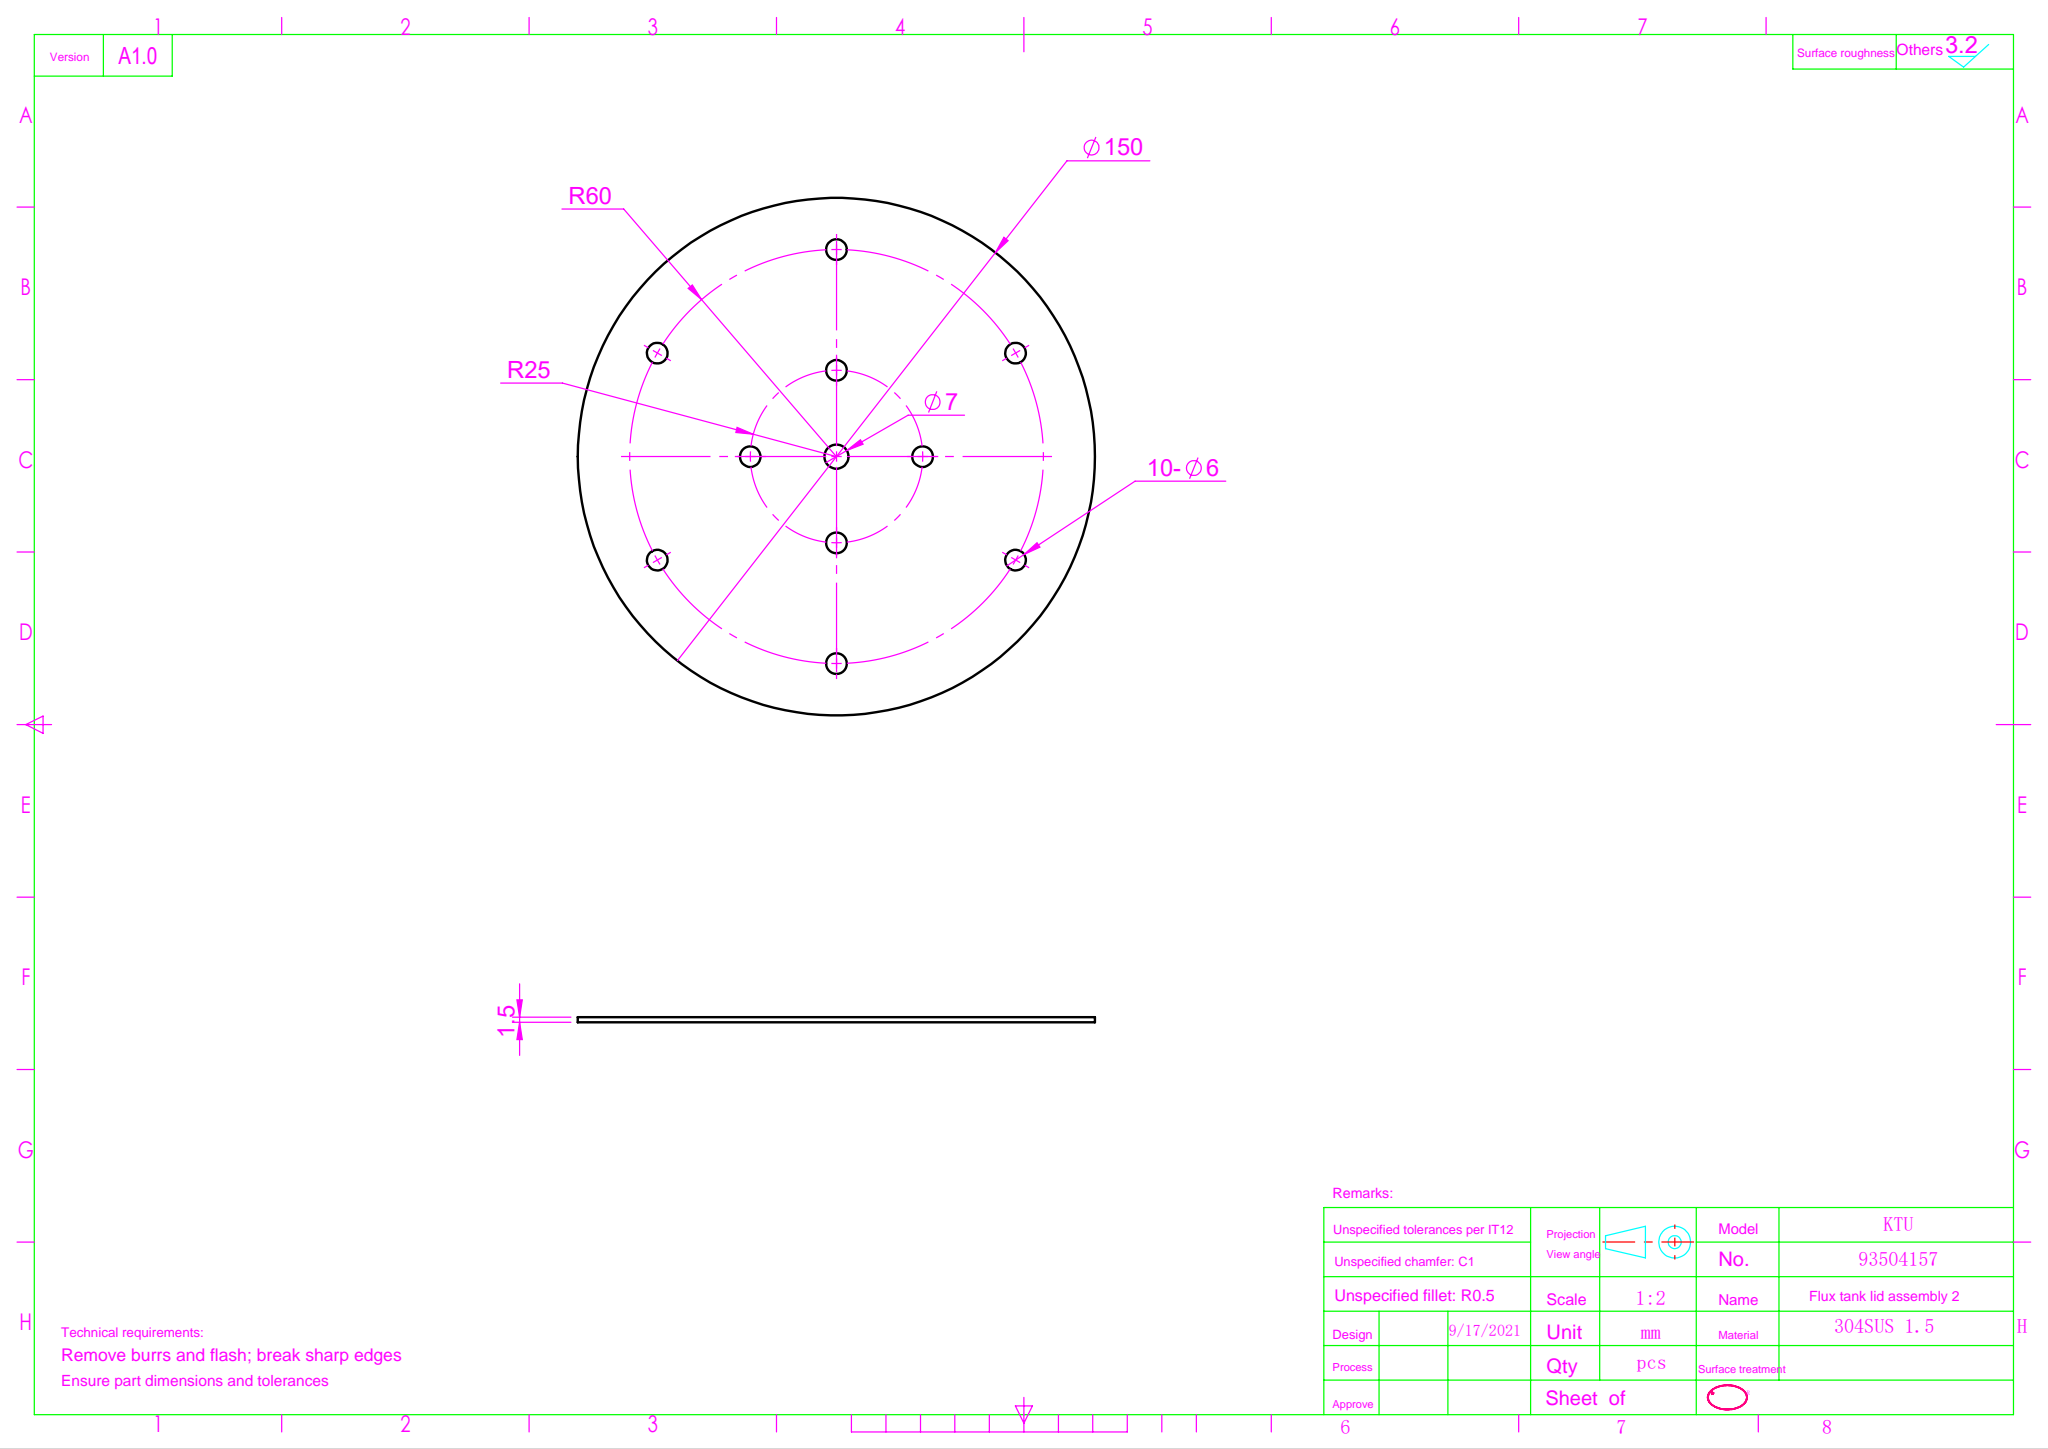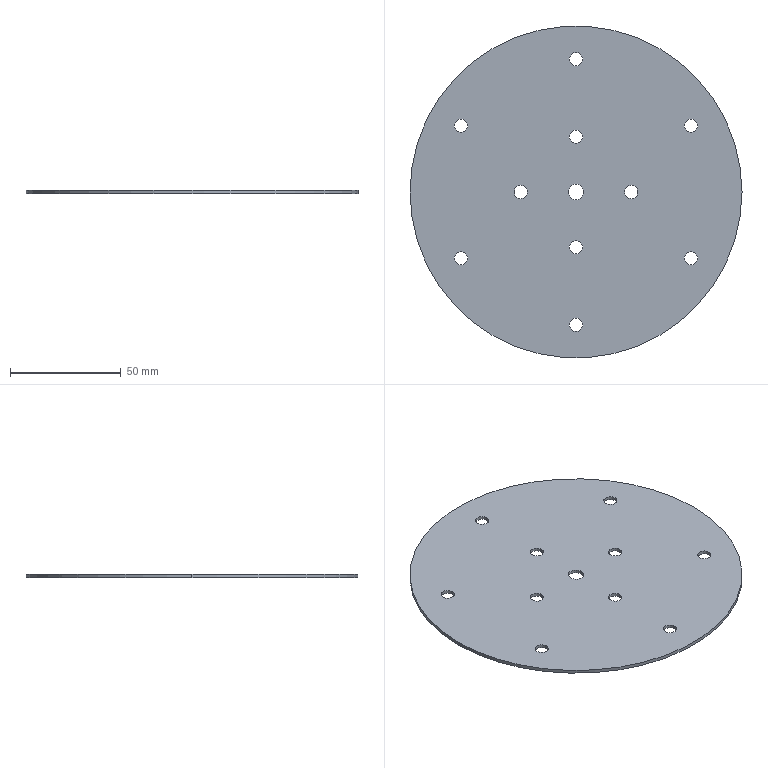Part | SolidWorks | features CirPattern 2, ICE 2, FlatPattern 1, HoleWzd 1, SMBaseFlange 1, SheetMetal 1 | 1 solid | 26 faces | box 150 x 150 x 1.5 mm | volume 26025 mm3 | cylinder 24 | plane 2 | commonest cylinder face diameters 6 x20 7 x2 150 x2
STEP:
#1=CARTESIAN_POINT('',(28.,0.,0.));
#2=VERTEX_POINT('',#1);
#3=CARTESIAN_POINT('',(22.,0.,0.));
#4=VERTEX_POINT('',#3);
#5=CARTESIAN_POINT('',(25.,0.,0.));
#6=DIRECTION('',(0.,0.,-1.));
#7=DIRECTION('',(1.,0.,0.));
#8=AXIS2_PLACEMENT_3D('',#5,#6,#7);
#9=CIRCLE('',#8,3.);
#10=EDGE_CURVE('',#2,#4,#9,.T.);
#11=ORIENTED_EDGE('',*,*,#10,.F.);
#12=CARTESIAN_POINT('',(28.,0.,-1.5));
#13=VERTEX_POINT('',#12);
#14=CARTESIAN_POINT('',(28.,0.,0.));
#15=DIRECTION('',(0.,0.,-1.));
#16=VECTOR('',#15,1000.);
#17=LINE('',#14,#16);
#18=EDGE_CURVE('',#2,#13,#17,.T.);
#19=ORIENTED_EDGE('',*,*,#18,.T.);
#20=CARTESIAN_POINT('',(22.,0.,-1.5));
#21=VERTEX_POINT('',#20);
#22=CARTESIAN_POINT('',(25.,0.,-1.5));
#23=DIRECTION('',(0.,0.,-1.));
#24=DIRECTION('',(1.,0.,0.));
#25=AXIS2_PLACEMENT_3D('',#22,#23,#24);
#26=CIRCLE('',#25,3.);
#27=EDGE_CURVE('',#13,#21,#26,.T.);
#28=ORIENTED_EDGE('',*,*,#27,.T.);
#29=CARTESIAN_POINT('',(22.,0.,0.));
#30=DIRECTION('',(0.,0.,-1.));
#31=VECTOR('',#30,1000.);
#32=LINE('',#29,#31);
#33=EDGE_CURVE('',#4,#21,#32,.T.);
#34=ORIENTED_EDGE('',*,*,#33,.F.);
#35=EDGE_LOOP('',(#11,#19,#28,#34));
#36=FACE_OUTER_BOUND('',#35,.T.);
#37=CARTESIAN_POINT('',(25.,0.,0.));
#38=DIRECTION('',(0.,0.,-1.));
#39=DIRECTION('',(-1.,0.,0.));
#40=AXIS2_PLACEMENT_3D('',#37,#38,#39);
#41=CYLINDRICAL_SURFACE('',#40,3.);
#42=ADVANCED_FACE('',(#36),#41,.F.);
#43=CARTESIAN_POINT('',(3.,25.,0.));
#44=VERTEX_POINT('',#43);
#45=CARTESIAN_POINT('',(-3.,25.,0.));
#46=VERTEX_POINT('',#45);
#47=CARTESIAN_POINT('',(0.,25.,0.));
#48=DIRECTION('',(0.,0.,-1.));
#49=DIRECTION('',(0.,1.,0.));
#50=AXIS2_PLACEMENT_3D('',#47,#48,#49);
#51=CIRCLE('',#50,3.);
#52=EDGE_CURVE('',#44,#46,#51,.T.);
#53=ORIENTED_EDGE('',*,*,#52,.F.);
#54=CARTESIAN_POINT('',(3.,25.,-1.5));
#55=VERTEX_POINT('',#54);
#56=CARTESIAN_POINT('',(3.,25.,0.));
#57=DIRECTION('',(0.,0.,-1.));
#58=VECTOR('',#57,1000.);
#59=LINE('',#56,#58);
#60=EDGE_CURVE('',#44,#55,#59,.T.);
#61=ORIENTED_EDGE('',*,*,#60,.T.);
#62=CARTESIAN_POINT('',(-3.,25.,-1.5));
#63=VERTEX_POINT('',#62);
#64=CARTESIAN_POINT('',(0.,25.,-1.5));
#65=DIRECTION('',(0.,0.,-1.));
#66=DIRECTION('',(0.,1.,0.));
#67=AXIS2_PLACEMENT_3D('',#64,#65,#66);
#68=CIRCLE('',#67,3.);
#69=EDGE_CURVE('',#55,#63,#68,.T.);
#70=ORIENTED_EDGE('',*,*,#69,.T.);
#71=CARTESIAN_POINT('',(-3.,25.,0.));
#72=DIRECTION('',(0.,0.,-1.));
#73=VECTOR('',#72,1000.);
#74=LINE('',#71,#73);
#75=EDGE_CURVE('',#46,#63,#74,.T.);
#76=ORIENTED_EDGE('',*,*,#75,.F.);
#77=EDGE_LOOP('',(#53,#61,#70,#76));
#78=FACE_OUTER_BOUND('',#77,.T.);
#79=CARTESIAN_POINT('',(0.,25.,0.));
#80=DIRECTION('',(0.,0.,-1.));
#81=DIRECTION('',(-1.,0.,0.));
#82=AXIS2_PLACEMENT_3D('',#79,#80,#81);
#83=CYLINDRICAL_SURFACE('',#82,3.);
#84=ADVANCED_FACE('',(#78),#83,.F.);
#85=CARTESIAN_POINT('',(3.,-25.,0.));
#86=VERTEX_POINT('',#85);
#87=CARTESIAN_POINT('',(-3.,-25.,0.));
#88=VERTEX_POINT('',#87);
#89=CARTESIAN_POINT('',(0.,-25.,0.));
#90=DIRECTION('',(0.,0.,-1.));
#91=DIRECTION('',(0.,-1.,0.));
#92=AXIS2_PLACEMENT_3D('',#89,#90,#91);
#93=CIRCLE('',#92,3.);
#94=EDGE_CURVE('',#86,#88,#93,.T.);
#95=ORIENTED_EDGE('',*,*,#94,.F.);
#96=CARTESIAN_POINT('',(3.,-25.,-1.5));
#97=VERTEX_POINT('',#96);
#98=CARTESIAN_POINT('',(3.,-25.,0.));
#99=DIRECTION('',(0.,0.,-1.));
#100=VECTOR('',#99,1000.);
#101=LINE('',#98,#100);
#102=EDGE_CURVE('',#86,#97,#101,.T.);
#103=ORIENTED_EDGE('',*,*,#102,.T.);
#104=CARTESIAN_POINT('',(-3.,-25.,-1.5));
#105=VERTEX_POINT('',#104);
#106=CARTESIAN_POINT('',(0.,-25.,-1.5));
#107=DIRECTION('',(0.,0.,-1.));
#108=DIRECTION('',(0.,-1.,0.));
#109=AXIS2_PLACEMENT_3D('',#106,#107,#108);
#110=CIRCLE('',#109,3.);
#111=EDGE_CURVE('',#97,#105,#110,.T.);
#112=ORIENTED_EDGE('',*,*,#111,.T.);
#113=CARTESIAN_POINT('',(-3.,-25.,0.));
#114=DIRECTION('',(0.,0.,-1.));
#115=VECTOR('',#114,1000.);
#116=LINE('',#113,#115);
#117=EDGE_CURVE('',#88,#105,#116,.T.);
#118=ORIENTED_EDGE('',*,*,#117,.F.);
#119=EDGE_LOOP('',(#95,#103,#112,#118));
#120=FACE_OUTER_BOUND('',#119,.T.);
#121=CARTESIAN_POINT('',(0.,-25.,0.));
#122=DIRECTION('',(0.,0.,-1.));
#123=DIRECTION('',(-1.,0.,0.));
#124=AXIS2_PLACEMENT_3D('',#121,#122,#123);
#125=CYLINDRICAL_SURFACE('',#124,3.);
#126=ADVANCED_FACE('',(#120),#125,.F.);
#127=CARTESIAN_POINT('',(-22.,0.,0.));
#128=VERTEX_POINT('',#127);
#129=CARTESIAN_POINT('',(-28.,0.,0.));
#130=VERTEX_POINT('',#129);
#131=CARTESIAN_POINT('',(-25.,0.,0.));
#132=DIRECTION('',(0.,0.,-1.));
#133=DIRECTION('',(-1.,0.,0.));
#134=AXIS2_PLACEMENT_3D('',#131,#132,#133);
#135=CIRCLE('',#134,3.);
#136=EDGE_CURVE('',#128,#130,#135,.T.);
#137=ORIENTED_EDGE('',*,*,#136,.F.);
#138=CARTESIAN_POINT('',(-22.,0.,-1.5));
#139=VERTEX_POINT('',#138);
#140=CARTESIAN_POINT('',(-22.,0.,0.));
#141=DIRECTION('',(0.,0.,-1.));
#142=VECTOR('',#141,1000.);
#143=LINE('',#140,#142);
#144=EDGE_CURVE('',#128,#139,#143,.T.);
#145=ORIENTED_EDGE('',*,*,#144,.T.);
#146=CARTESIAN_POINT('',(-28.,0.,-1.5));
#147=VERTEX_POINT('',#146);
#148=CARTESIAN_POINT('',(-25.,0.,-1.5));
#149=DIRECTION('',(0.,0.,-1.));
#150=DIRECTION('',(-1.,0.,0.));
#151=AXIS2_PLACEMENT_3D('',#148,#149,#150);
#152=CIRCLE('',#151,3.);
#153=EDGE_CURVE('',#139,#147,#152,.T.);
#154=ORIENTED_EDGE('',*,*,#153,.T.);
#155=CARTESIAN_POINT('',(-28.,0.,0.));
#156=DIRECTION('',(0.,0.,-1.));
#157=VECTOR('',#156,1000.);
#158=LINE('',#155,#157);
#159=EDGE_CURVE('',#130,#147,#158,.T.);
#160=ORIENTED_EDGE('',*,*,#159,.F.);
#161=EDGE_LOOP('',(#137,#145,#154,#160));
#162=FACE_OUTER_BOUND('',#161,.T.);
#163=CARTESIAN_POINT('',(-25.,0.,0.));
#164=DIRECTION('',(0.,0.,-1.));
#165=DIRECTION('',(-1.,0.,0.));
#166=AXIS2_PLACEMENT_3D('',#163,#164,#165);
#167=CYLINDRICAL_SURFACE('',#166,3.);
#168=ADVANCED_FACE('',(#162),#167,.F.);
#169=CARTESIAN_POINT('',(-48.962,-30.,0.));
#170=VERTEX_POINT('',#169);
#171=CARTESIAN_POINT('',(-54.962,-30.,0.));
#172=VERTEX_POINT('',#171);
#173=CARTESIAN_POINT('',(-51.962,-30.,0.));
#174=DIRECTION('',(0.,0.,-1.));
#175=DIRECTION('',(1.,0.,0.));
#176=AXIS2_PLACEMENT_3D('',#173,#174,#175);
#177=CIRCLE('',#176,3.);
#178=EDGE_CURVE('',#170,#172,#177,.T.);
#179=ORIENTED_EDGE('',*,*,#178,.F.);
#180=CARTESIAN_POINT('',(-48.962,-30.,-1.5));
#181=VERTEX_POINT('',#180);
#182=CARTESIAN_POINT('',(-48.962,-30.,0.001));
#183=DIRECTION('',(0.,0.,-1.));
#184=VECTOR('',#183,1000.);
#185=LINE('',#182,#184);
#186=EDGE_CURVE('',#170,#181,#185,.T.);
#187=ORIENTED_EDGE('',*,*,#186,.T.);
#188=CARTESIAN_POINT('',(-54.962,-30.,-1.5));
#189=VERTEX_POINT('',#188);
#190=CARTESIAN_POINT('',(-51.962,-30.,-1.5));
#191=DIRECTION('',(0.,0.,-1.));
#192=DIRECTION('',(0.5,-0.866,0.));
#193=AXIS2_PLACEMENT_3D('',#190,#191,#192);
#194=CIRCLE('',#193,3.);
#195=EDGE_CURVE('',#181,#189,#194,.T.);
#196=ORIENTED_EDGE('',*,*,#195,.T.);
#197=CARTESIAN_POINT('',(-54.962,-30.,0.001));
#198=DIRECTION('',(0.,0.,-1.));
#199=VECTOR('',#198,1000.);
#200=LINE('',#197,#199);
#201=EDGE_CURVE('',#172,#189,#200,.T.);
#202=ORIENTED_EDGE('',*,*,#201,.F.);
#203=EDGE_LOOP('',(#179,#187,#196,#202));
#204=FACE_OUTER_BOUND('',#203,.T.);
#205=CARTESIAN_POINT('',(-51.962,-30.,0.001));
#206=DIRECTION('',(0.,0.,-1.));
#207=DIRECTION('',(-1.,0.,0.));
#208=AXIS2_PLACEMENT_3D('',#205,#206,#207);
#209=CYLINDRICAL_SURFACE('',#208,3.);
#210=ADVANCED_FACE('',(#204),#209,.F.);
#211=CARTESIAN_POINT('',(3.,-60.,0.));
#212=VERTEX_POINT('',#211);
#213=CARTESIAN_POINT('',(-3.,-60.,0.));
#214=VERTEX_POINT('',#213);
#215=CARTESIAN_POINT('',(0.,-60.,0.));
#216=DIRECTION('',(0.,0.,-1.));
#217=DIRECTION('',(1.,0.,0.));
#218=AXIS2_PLACEMENT_3D('',#215,#216,#217);
#219=CIRCLE('',#218,3.);
#220=EDGE_CURVE('',#212,#214,#219,.T.);
#221=ORIENTED_EDGE('',*,*,#220,.F.);
#222=CARTESIAN_POINT('',(3.,-60.,-1.5));
#223=VERTEX_POINT('',#222);
#224=CARTESIAN_POINT('',(3.,-60.,0.001));
#225=DIRECTION('',(0.,0.,-1.));
#226=VECTOR('',#225,1000.);
#227=LINE('',#224,#226);
#228=EDGE_CURVE('',#212,#223,#227,.T.);
#229=ORIENTED_EDGE('',*,*,#228,.T.);
#230=CARTESIAN_POINT('',(-3.,-60.,-1.5));
#231=VERTEX_POINT('',#230);
#232=CARTESIAN_POINT('',(0.,-60.,-1.5));
#233=DIRECTION('',(0.,0.,-1.));
#234=DIRECTION('',(1.,0.,0.));
#235=AXIS2_PLACEMENT_3D('',#232,#233,#234);
#236=CIRCLE('',#235,3.);
#237=EDGE_CURVE('',#223,#231,#236,.T.);
#238=ORIENTED_EDGE('',*,*,#237,.T.);
#239=CARTESIAN_POINT('',(-3.,-60.,0.001));
#240=DIRECTION('',(0.,0.,-1.));
#241=VECTOR('',#240,1000.);
#242=LINE('',#239,#241);
#243=EDGE_CURVE('',#214,#231,#242,.T.);
#244=ORIENTED_EDGE('',*,*,#243,.F.);
#245=EDGE_LOOP('',(#221,#229,#238,#244));
#246=FACE_OUTER_BOUND('',#245,.T.);
#247=CARTESIAN_POINT('',(0.,-60.,0.001));
#248=DIRECTION('',(0.,0.,-1.));
#249=DIRECTION('',(-1.,0.,0.));
#250=AXIS2_PLACEMENT_3D('',#247,#248,#249);
#251=CYLINDRICAL_SURFACE('',#250,3.);
#252=ADVANCED_FACE('',(#246),#251,.F.);
#253=CARTESIAN_POINT('',(54.962,-30.,0.));
#254=VERTEX_POINT('',#253);
#255=CARTESIAN_POINT('',(48.962,-30.,0.));
#256=VERTEX_POINT('',#255);
#257=CARTESIAN_POINT('',(51.962,-30.,0.));
#258=DIRECTION('',(0.,0.,-1.));
#259=DIRECTION('',(1.,0.,0.));
#260=AXIS2_PLACEMENT_3D('',#257,#258,#259);
#261=CIRCLE('',#260,3.);
#262=EDGE_CURVE('',#254,#256,#261,.T.);
#263=ORIENTED_EDGE('',*,*,#262,.F.);
#264=CARTESIAN_POINT('',(54.962,-30.,-1.5));
#265=VERTEX_POINT('',#264);
#266=CARTESIAN_POINT('',(54.962,-30.,0.001));
#267=DIRECTION('',(0.,0.,-1.));
#268=VECTOR('',#267,1000.);
#269=LINE('',#266,#268);
#270=EDGE_CURVE('',#254,#265,#269,.T.);
#271=ORIENTED_EDGE('',*,*,#270,.T.);
#272=CARTESIAN_POINT('',(48.962,-30.,-1.5));
#273=VERTEX_POINT('',#272);
#274=CARTESIAN_POINT('',(51.962,-30.,-1.5));
#275=DIRECTION('',(0.,0.,-1.));
#276=DIRECTION('',(0.5,0.866,0.));
#277=AXIS2_PLACEMENT_3D('',#274,#275,#276);
#278=CIRCLE('',#277,3.);
#279=EDGE_CURVE('',#265,#273,#278,.T.);
#280=ORIENTED_EDGE('',*,*,#279,.T.);
#281=CARTESIAN_POINT('',(48.962,-30.,0.001));
#282=DIRECTION('',(0.,0.,-1.));
#283=VECTOR('',#282,1000.);
#284=LINE('',#281,#283);
#285=EDGE_CURVE('',#256,#273,#284,.T.);
#286=ORIENTED_EDGE('',*,*,#285,.F.);
#287=EDGE_LOOP('',(#263,#271,#280,#286));
#288=FACE_OUTER_BOUND('',#287,.T.);
#289=CARTESIAN_POINT('',(51.962,-30.,0.001));
#290=DIRECTION('',(0.,0.,-1.));
#291=DIRECTION('',(-1.,0.,0.));
#292=AXIS2_PLACEMENT_3D('',#289,#290,#291);
#293=CYLINDRICAL_SURFACE('',#292,3.);
#294=ADVANCED_FACE('',(#288),#293,.F.);
#295=CARTESIAN_POINT('',(54.962,30.,0.));
#296=VERTEX_POINT('',#295);
#297=CARTESIAN_POINT('',(48.962,30.,0.));
#298=VERTEX_POINT('',#297);
#299=CARTESIAN_POINT('',(51.962,30.,0.));
#300=DIRECTION('',(0.,0.,-1.));
#301=DIRECTION('',(1.,0.,0.));
#302=AXIS2_PLACEMENT_3D('',#299,#300,#301);
#303=CIRCLE('',#302,3.);
#304=EDGE_CURVE('',#296,#298,#303,.T.);
#305=ORIENTED_EDGE('',*,*,#304,.F.);
#306=CARTESIAN_POINT('',(54.962,30.,-1.5));
#307=VERTEX_POINT('',#306);
#308=CARTESIAN_POINT('',(54.962,30.,0.001));
#309=DIRECTION('',(0.,0.,-1.));
#310=VECTOR('',#309,1000.);
#311=LINE('',#308,#310);
#312=EDGE_CURVE('',#296,#307,#311,.T.);
#313=ORIENTED_EDGE('',*,*,#312,.T.);
#314=CARTESIAN_POINT('',(48.962,30.,-1.5));
#315=VERTEX_POINT('',#314);
#316=CARTESIAN_POINT('',(51.962,30.,-1.5));
#317=DIRECTION('',(0.,0.,-1.));
#318=DIRECTION('',(-0.5,0.866,0.));
#319=AXIS2_PLACEMENT_3D('',#316,#317,#318);
#320=CIRCLE('',#319,3.);
#321=EDGE_CURVE('',#307,#315,#320,.T.);
#322=ORIENTED_EDGE('',*,*,#321,.T.);
#323=CARTESIAN_POINT('',(48.962,30.,0.001));
#324=DIRECTION('',(0.,0.,-1.));
#325=VECTOR('',#324,1000.);
#326=LINE('',#323,#325);
#327=EDGE_CURVE('',#298,#315,#326,.T.);
#328=ORIENTED_EDGE('',*,*,#327,.F.);
#329=EDGE_LOOP('',(#305,#313,#322,#328));
#330=FACE_OUTER_BOUND('',#329,.T.);
#331=CARTESIAN_POINT('',(51.962,30.,0.001));
#332=DIRECTION('',(0.,0.,-1.));
#333=DIRECTION('',(-1.,0.,0.));
#334=AXIS2_PLACEMENT_3D('',#331,#332,#333);
#335=CYLINDRICAL_SURFACE('',#334,3.);
#336=ADVANCED_FACE('',(#330),#335,.F.);
#337=CARTESIAN_POINT('',(-48.962,30.,0.));
#338=VERTEX_POINT('',#337);
#339=CARTESIAN_POINT('',(-54.962,30.,0.));
#340=VERTEX_POINT('',#339);
#341=CARTESIAN_POINT('',(-51.962,30.,0.));
#342=DIRECTION('',(0.,0.,-1.));
#343=DIRECTION('',(1.,0.,0.));
#344=AXIS2_PLACEMENT_3D('',#341,#342,#343);
#345=CIRCLE('',#344,3.);
#346=EDGE_CURVE('',#338,#340,#345,.T.);
#347=ORIENTED_EDGE('',*,*,#346,.F.);
#348=CARTESIAN_POINT('',(-48.962,30.,-1.5));
#349=VERTEX_POINT('',#348);
#350=CARTESIAN_POINT('',(-48.962,30.,0.001));
#351=DIRECTION('',(0.,0.,-1.));
#352=VECTOR('',#351,1000.);
#353=LINE('',#350,#352);
#354=EDGE_CURVE('',#338,#349,#353,.T.);
#355=ORIENTED_EDGE('',*,*,#354,.T.);
#356=CARTESIAN_POINT('',(-54.962,30.,-1.5));
#357=VERTEX_POINT('',#356);
#358=CARTESIAN_POINT('',(-51.962,30.,-1.5));
#359=DIRECTION('',(0.,0.,-1.));
#360=DIRECTION('',(-0.5,-0.866,0.));
#361=AXIS2_PLACEMENT_3D('',#358,#359,#360);
#362=CIRCLE('',#361,3.);
#363=EDGE_CURVE('',#349,#357,#362,.T.);
#364=ORIENTED_EDGE('',*,*,#363,.T.);
#365=CARTESIAN_POINT('',(-54.962,30.,0.001));
#366=DIRECTION('',(0.,0.,-1.));
#367=VECTOR('',#366,1000.);
#368=LINE('',#365,#367);
#369=EDGE_CURVE('',#340,#357,#368,.T.);
#370=ORIENTED_EDGE('',*,*,#369,.F.);
#371=EDGE_LOOP('',(#347,#355,#364,#370));
#372=FACE_OUTER_BOUND('',#371,.T.);
#373=CARTESIAN_POINT('',(-51.962,30.,0.001));
#374=DIRECTION('',(0.,0.,-1.));
#375=DIRECTION('',(-1.,0.,0.));
#376=AXIS2_PLACEMENT_3D('',#373,#374,#375);
#377=CYLINDRICAL_SURFACE('',#376,3.);
#378=ADVANCED_FACE('',(#372),#377,.F.);
#379=CARTESIAN_POINT('',(3.,60.,0.));
#380=VERTEX_POINT('',#379);
#381=CARTESIAN_POINT('',(-3.,60.,0.));
#382=VERTEX_POINT('',#381);
#383=CARTESIAN_POINT('',(0.,60.,0.));
#384=DIRECTION('',(0.,0.,-1.));
#385=DIRECTION('',(1.,0.,0.));
#386=AXIS2_PLACEMENT_3D('',#383,#384,#385);
#387=CIRCLE('',#386,3.);
#388=EDGE_CURVE('',#380,#382,#387,.T.);
#389=ORIENTED_EDGE('',*,*,#388,.F.);
#390=CARTESIAN_POINT('',(3.,60.,-1.5));
#391=VERTEX_POINT('',#390);
#392=CARTESIAN_POINT('',(3.,60.,0.001));
#393=DIRECTION('',(0.,0.,-1.));
#394=VECTOR('',#393,1000.);
#395=LINE('',#392,#394);
#396=EDGE_CURVE('',#380,#391,#395,.T.);
#397=ORIENTED_EDGE('',*,*,#396,.T.);
#398=CARTESIAN_POINT('',(-3.,60.,-1.5));
#399=VERTEX_POINT('',#398);
#400=CARTESIAN_POINT('',(0.,60.,-1.5));
#401=DIRECTION('',(0.,0.,-1.));
#402=DIRECTION('',(-1.,0.,0.));
#403=AXIS2_PLACEMENT_3D('',#400,#401,#402);
#404=CIRCLE('',#403,3.);
#405=EDGE_CURVE('',#391,#399,#404,.T.);
#406=ORIENTED_EDGE('',*,*,#405,.T.);
#407=CARTESIAN_POINT('',(-3.,60.,0.001));
#408=DIRECTION('',(0.,0.,-1.));
#409=VECTOR('',#408,1000.);
#410=LINE('',#407,#409);
#411=EDGE_CURVE('',#382,#399,#410,.T.);
#412=ORIENTED_EDGE('',*,*,#411,.F.);
#413=EDGE_LOOP('',(#389,#397,#406,#412));
#414=FACE_OUTER_BOUND('',#413,.T.);
#415=CARTESIAN_POINT('',(0.,60.,0.001));
#416=DIRECTION('',(0.,0.,-1.));
#417=DIRECTION('',(-1.,0.,0.));
#418=AXIS2_PLACEMENT_3D('',#415,#416,#417);
#419=CYLINDRICAL_SURFACE('',#418,3.);
#420=ADVANCED_FACE('',(#414),#419,.F.);
#421=CARTESIAN_POINT('',(-3.5,0.,0.));
#422=VERTEX_POINT('',#421);
#423=CARTESIAN_POINT('',(3.5,0.,0.));
#424=VERTEX_POINT('',#423);
#425=CARTESIAN_POINT('',(0.,0.,0.));
#426=DIRECTION('',(0.,0.,1.));
#427=DIRECTION('',(1.,0.,0.));
#428=AXIS2_PLACEMENT_3D('',#425,#426,#427);
#429=CIRCLE('',#428,3.5);
#430=EDGE_CURVE('',#422,#424,#429,.T.);
#431=ORIENTED_EDGE('',*,*,#430,.T.);
#432=CARTESIAN_POINT('',(3.5,0.,-1.5));
#433=VERTEX_POINT('',#432);
#434=CARTESIAN_POINT('',(3.5,0.,-1.5));
#435=DIRECTION('',(0.,0.,-1.));
#436=VECTOR('',#435,1000.);
#437=LINE('',#434,#436);
#438=EDGE_CURVE('',#424,#433,#437,.T.);
#439=ORIENTED_EDGE('',*,*,#438,.T.);
#440=CARTESIAN_POINT('',(-3.5,0.,-1.5));
#441=VERTEX_POINT('',#440);
#442=CARTESIAN_POINT('',(0.,0.,-1.5));
#443=DIRECTION('',(0.,0.,-1.));
#444=DIRECTION('',(-1.,0.,0.));
#445=AXIS2_PLACEMENT_3D('',#442,#443,#444);
#446=CIRCLE('',#445,3.5);
#447=EDGE_CURVE('',#433,#441,#446,.T.);
#448=ORIENTED_EDGE('',*,*,#447,.T.);
#449=CARTESIAN_POINT('',(-3.5,0.,-1.5));
#450=DIRECTION('',(0.,0.,-1.));
#451=VECTOR('',#450,1000.);
#452=LINE('',#449,#451);
#453=EDGE_CURVE('',#422,#441,#452,.T.);
#454=ORIENTED_EDGE('',*,*,#453,.F.);
#455=EDGE_LOOP('',(#431,#439,#448,#454));
#456=FACE_OUTER_BOUND('',#455,.T.);
#457=CARTESIAN_POINT('',(0.,0.,-1.5));
#458=DIRECTION('',(0.,0.,-1.));
#459=DIRECTION('',(-1.,0.,0.));
#460=AXIS2_PLACEMENT_3D('',#457,#458,#459);
#461=CYLINDRICAL_SURFACE('',#460,3.5);
#462=ADVANCED_FACE('',(#456),#461,.F.);
#463=CARTESIAN_POINT('',(75.,0.,-1.5));
#464=VERTEX_POINT('',#463);
#465=CARTESIAN_POINT('',(-75.,0.,-1.5));
#466=VERTEX_POINT('',#465);
#467=CARTESIAN_POINT('',(0.,0.,-1.5));
#468=DIRECTION('',(0.,0.,1.));
#469=DIRECTION('',(1.,0.,0.));
#470=AXIS2_PLACEMENT_3D('',#467,#468,#469);
#471=CIRCLE('',#470,75.);
#472=EDGE_CURVE('',#464,#466,#471,.T.);
#473=ORIENTED_EDGE('',*,*,#472,.T.);
#474=CARTESIAN_POINT('',(-75.,0.,0.));
#475=VERTEX_POINT('',#474);
#476=CARTESIAN_POINT('',(-75.,0.,-1.5));
#477=DIRECTION('',(0.,0.,1.));
#478=VECTOR('',#477,1000.);
#479=LINE('',#476,#478);
#480=EDGE_CURVE('',#466,#475,#479,.T.);
#481=ORIENTED_EDGE('',*,*,#480,.T.);
#482=CARTESIAN_POINT('',(75.,0.,0.));
#483=VERTEX_POINT('',#482);
#484=CARTESIAN_POINT('',(0.,0.,0.));
#485=DIRECTION('',(0.,0.,1.));
#486=DIRECTION('',(1.,0.,0.));
#487=AXIS2_PLACEMENT_3D('',#484,#485,#486);
#488=CIRCLE('',#487,75.);
#489=EDGE_CURVE('',#483,#475,#488,.T.);
#490=ORIENTED_EDGE('',*,*,#489,.F.);
#491=CARTESIAN_POINT('',(75.,0.,-1.5));
#492=DIRECTION('',(0.,0.,1.));
#493=VECTOR('',#492,1000.);
#494=LINE('',#491,#493);
#495=EDGE_CURVE('',#464,#483,#494,.T.);
#496=ORIENTED_EDGE('',*,*,#495,.F.);
#497=EDGE_LOOP('',(#473,#481,#490,#496));
#498=FACE_OUTER_BOUND('',#497,.T.);
#499=CARTESIAN_POINT('',(0.,0.,-1.5));
#500=DIRECTION('',(0.,0.,1.));
#501=DIRECTION('',(1.,0.,0.));
#502=AXIS2_PLACEMENT_3D('',#499,#500,#501);
#503=CYLINDRICAL_SURFACE('',#502,75.);
#504=ADVANCED_FACE('',(#498),#503,.T.);
#505=ORIENTED_EDGE('',*,*,#480,.F.);
#506=CARTESIAN_POINT('',(0.,0.,-1.5));
#507=DIRECTION('',(0.,0.,1.));
#508=DIRECTION('',(1.,0.,0.));
#509=AXIS2_PLACEMENT_3D('',#506,#507,#508);
#510=CIRCLE('',#509,75.);
#511=EDGE_CURVE('',#466,#464,#510,.T.);
#512=ORIENTED_EDGE('',*,*,#511,.T.);
#513=ORIENTED_EDGE('',*,*,#495,.T.);
#514=CARTESIAN_POINT('',(0.,0.,0.));
#515=DIRECTION('',(0.,0.,1.));
#516=DIRECTION('',(1.,0.,0.));
#517=AXIS2_PLACEMENT_3D('',#514,#515,#516);
#518=CIRCLE('',#517,75.);
#519=EDGE_CURVE('',#475,#483,#518,.T.);
#520=ORIENTED_EDGE('',*,*,#519,.F.);
#521=EDGE_LOOP('',(#505,#512,#513,#520));
#522=FACE_OUTER_BOUND('',#521,.T.);
#523=CARTESIAN_POINT('',(0.,0.,-1.5));
#524=DIRECTION('',(0.,0.,1.));
#525=DIRECTION('',(1.,0.,0.));
#526=AXIS2_PLACEMENT_3D('',#523,#524,#525);
#527=CYLINDRICAL_SURFACE('',#526,75.);
#528=ADVANCED_FACE('',(#522),#527,.T.);
#529=CARTESIAN_POINT('',(25.,0.,-1.5));
#530=DIRECTION('',(0.,0.,-1.));
#531=DIRECTION('',(1.,0.,0.));
#532=AXIS2_PLACEMENT_3D('',#529,#530,#531);
#533=CIRCLE('',#532,3.);
#534=EDGE_CURVE('',#21,#13,#533,.T.);
#535=ORIENTED_EDGE('',*,*,#534,.F.);
#536=ORIENTED_EDGE('',*,*,#27,.F.);
#537=EDGE_LOOP('',(#535,#536));
#538=FACE_BOUND('',#537,.T.);
#539=CARTESIAN_POINT('',(0.,25.,-1.5));
#540=DIRECTION('',(0.,0.,-1.));
#541=DIRECTION('',(0.,1.,0.));
#542=AXIS2_PLACEMENT_3D('',#539,#540,#541);
#543=CIRCLE('',#542,3.);
#544=EDGE_CURVE('',#63,#55,#543,.T.);
#545=ORIENTED_EDGE('',*,*,#544,.F.);
#546=ORIENTED_EDGE('',*,*,#69,.F.);
#547=EDGE_LOOP('',(#545,#546));
#548=FACE_BOUND('',#547,.T.);
#549=CARTESIAN_POINT('',(0.,-25.,-1.5));
#550=DIRECTION('',(0.,0.,-1.));
#551=DIRECTION('',(0.,-1.,0.));
#552=AXIS2_PLACEMENT_3D('',#549,#550,#551);
#553=CIRCLE('',#552,3.);
#554=EDGE_CURVE('',#105,#97,#553,.T.);
#555=ORIENTED_EDGE('',*,*,#554,.F.);
#556=ORIENTED_EDGE('',*,*,#111,.F.);
#557=EDGE_LOOP('',(#555,#556));
#558=FACE_BOUND('',#557,.T.);
#559=CARTESIAN_POINT('',(-25.,0.,-1.5));
#560=DIRECTION('',(0.,0.,-1.));
#561=DIRECTION('',(-1.,0.,0.));
#562=AXIS2_PLACEMENT_3D('',#559,#560,#561);
#563=CIRCLE('',#562,3.);
#564=EDGE_CURVE('',#147,#139,#563,.T.);
#565=ORIENTED_EDGE('',*,*,#564,.F.);
#566=ORIENTED_EDGE('',*,*,#153,.F.);
#567=EDGE_LOOP('',(#565,#566));
#568=FACE_BOUND('',#567,.T.);
#569=CARTESIAN_POINT('',(-51.962,-30.,-1.5));
#570=DIRECTION('',(0.,0.,-1.));
#571=DIRECTION('',(0.5,-0.866,0.));
#572=AXIS2_PLACEMENT_3D('',#569,#570,#571);
#573=CIRCLE('',#572,3.);
#574=EDGE_CURVE('',#189,#181,#573,.T.);
#575=ORIENTED_EDGE('',*,*,#574,.F.);
#576=ORIENTED_EDGE('',*,*,#195,.F.);
#577=EDGE_LOOP('',(#575,#576));
#578=FACE_BOUND('',#577,.T.);
#579=CARTESIAN_POINT('',(0.,-60.,-1.5));
#580=DIRECTION('',(0.,0.,-1.));
#581=DIRECTION('',(1.,0.,0.));
#582=AXIS2_PLACEMENT_3D('',#579,#580,#581);
#583=CIRCLE('',#582,3.);
#584=EDGE_CURVE('',#231,#223,#583,.T.);
#585=ORIENTED_EDGE('',*,*,#584,.F.);
#586=ORIENTED_EDGE('',*,*,#237,.F.);
#587=EDGE_LOOP('',(#585,#586));
#588=FACE_BOUND('',#587,.T.);
#589=CARTESIAN_POINT('',(51.962,-30.,-1.5));
#590=DIRECTION('',(0.,0.,-1.));
#591=DIRECTION('',(0.5,0.866,0.));
#592=AXIS2_PLACEMENT_3D('',#589,#590,#591);
#593=CIRCLE('',#592,3.);
#594=EDGE_CURVE('',#273,#265,#593,.T.);
#595=ORIENTED_EDGE('',*,*,#594,.F.);
#596=ORIENTED_EDGE('',*,*,#279,.F.);
#597=EDGE_LOOP('',(#595,#596));
#598=FACE_BOUND('',#597,.T.);
#599=CARTESIAN_POINT('',(51.962,30.,-1.5));
#600=DIRECTION('',(0.,0.,-1.));
#601=DIRECTION('',(-0.5,0.866,0.));
#602=AXIS2_PLACEMENT_3D('',#599,#600,#601);
#603=CIRCLE('',#602,3.);
#604=EDGE_CURVE('',#315,#307,#603,.T.);
#605=ORIENTED_EDGE('',*,*,#604,.F.);
#606=ORIENTED_EDGE('',*,*,#321,.F.);
#607=EDGE_LOOP('',(#605,#606));
#608=FACE_BOUND('',#607,.T.);
#609=CARTESIAN_POINT('',(-51.962,30.,-1.5));
#610=DIRECTION('',(0.,0.,-1.));
#611=DIRECTION('',(-0.5,-0.866,0.));
#612=AXIS2_PLACEMENT_3D('',#609,#610,#611);
#613=CIRCLE('',#612,3.);
#614=EDGE_CURVE('',#357,#349,#613,.T.);
#615=ORIENTED_EDGE('',*,*,#614,.F.);
#616=ORIENTED_EDGE('',*,*,#363,.F.);
#617=EDGE_LOOP('',(#615,#616));
#618=FACE_BOUND('',#617,.T.);
#619=CARTESIAN_POINT('',(0.,60.,-1.5));
#620=DIRECTION('',(0.,0.,-1.));
#621=DIRECTION('',(-1.,0.,0.));
#622=AXIS2_PLACEMENT_3D('',#619,#620,#621);
#623=CIRCLE('',#622,3.);
#624=EDGE_CURVE('',#399,#391,#623,.T.);
#625=ORIENTED_EDGE('',*,*,#624,.F.);
#626=ORIENTED_EDGE('',*,*,#405,.F.);
#627=EDGE_LOOP('',(#625,#626));
#628=FACE_BOUND('',#627,.T.);
#629=CARTESIAN_POINT('',(0.,0.,-1.5));
#630=DIRECTION('',(0.,0.,-1.));
#631=DIRECTION('',(-1.,0.,0.));
#632=AXIS2_PLACEMENT_3D('',#629,#630,#631);
#633=CIRCLE('',#632,3.5);
#634=EDGE_CURVE('',#441,#433,#633,.T.);
#635=ORIENTED_EDGE('',*,*,#634,.F.);
#636=ORIENTED_EDGE('',*,*,#447,.F.);
#637=EDGE_LOOP('',(#635,#636));
#638=FACE_BOUND('',#637,.T.);
#639=ORIENTED_EDGE('',*,*,#472,.F.);
#640=ORIENTED_EDGE('',*,*,#511,.F.);
#641=EDGE_LOOP('',(#639,#640));
#642=FACE_OUTER_BOUND('',#641,.T.);
#643=CARTESIAN_POINT('',(0.,0.,-1.5));
#644=DIRECTION('',(0.,0.,1.));
#645=DIRECTION('',(1.,0.,0.));
#646=AXIS2_PLACEMENT_3D('',#643,#644,#645);
#647=PLANE('',#646);
#648=ADVANCED_FACE('',(#538,#548,#558,#568,#578,#588,#598,#608,#618,#628,#638,#642),#647,.F.);
#649=CARTESIAN_POINT('',(25.,0.,0.));
#650=DIRECTION('',(0.,0.,-1.));
#651=DIRECTION('',(1.,0.,0.));
#652=AXIS2_PLACEMENT_3D('',#649,#650,#651);
#653=CIRCLE('',#652,3.);
#654=EDGE_CURVE('',#4,#2,#653,.T.);
#655=ORIENTED_EDGE('',*,*,#654,.T.);
#656=ORIENTED_EDGE('',*,*,#10,.T.);
#657=EDGE_LOOP('',(#655,#656));
#658=FACE_BOUND('',#657,.T.);
#659=CARTESIAN_POINT('',(0.,25.,0.));
#660=DIRECTION('',(0.,0.,-1.));
#661=DIRECTION('',(0.,1.,0.));
#662=AXIS2_PLACEMENT_3D('',#659,#660,#661);
#663=CIRCLE('',#662,3.);
#664=EDGE_CURVE('',#46,#44,#663,.T.);
#665=ORIENTED_EDGE('',*,*,#664,.T.);
#666=ORIENTED_EDGE('',*,*,#52,.T.);
#667=EDGE_LOOP('',(#665,#666));
#668=FACE_BOUND('',#667,.T.);
#669=CARTESIAN_POINT('',(0.,-25.,0.));
#670=DIRECTION('',(0.,0.,-1.));
#671=DIRECTION('',(0.,-1.,0.));
#672=AXIS2_PLACEMENT_3D('',#669,#670,#671);
#673=CIRCLE('',#672,3.);
#674=EDGE_CURVE('',#88,#86,#673,.T.);
#675=ORIENTED_EDGE('',*,*,#674,.T.);
#676=ORIENTED_EDGE('',*,*,#94,.T.);
#677=EDGE_LOOP('',(#675,#676));
#678=FACE_BOUND('',#677,.T.);
#679=CARTESIAN_POINT('',(-25.,0.,0.));
#680=DIRECTION('',(0.,0.,-1.));
#681=DIRECTION('',(-1.,0.,0.));
#682=AXIS2_PLACEMENT_3D('',#679,#680,#681);
#683=CIRCLE('',#682,3.);
#684=EDGE_CURVE('',#130,#128,#683,.T.);
#685=ORIENTED_EDGE('',*,*,#684,.T.);
#686=ORIENTED_EDGE('',*,*,#136,.T.);
#687=EDGE_LOOP('',(#685,#686));
#688=FACE_BOUND('',#687,.T.);
#689=CARTESIAN_POINT('',(-51.962,-30.,0.));
#690=DIRECTION('',(0.,0.,-1.));
#691=DIRECTION('',(1.,0.,0.));
#692=AXIS2_PLACEMENT_3D('',#689,#690,#691);
#693=CIRCLE('',#692,3.);
#694=EDGE_CURVE('',#172,#170,#693,.T.);
#695=ORIENTED_EDGE('',*,*,#694,.T.);
#696=ORIENTED_EDGE('',*,*,#178,.T.);
#697=EDGE_LOOP('',(#695,#696));
#698=FACE_BOUND('',#697,.T.);
#699=CARTESIAN_POINT('',(0.,-60.,0.));
#700=DIRECTION('',(0.,0.,-1.));
#701=DIRECTION('',(1.,0.,0.));
#702=AXIS2_PLACEMENT_3D('',#699,#700,#701);
#703=CIRCLE('',#702,3.);
#704=EDGE_CURVE('',#214,#212,#703,.T.);
#705=ORIENTED_EDGE('',*,*,#704,.T.);
#706=ORIENTED_EDGE('',*,*,#220,.T.);
#707=EDGE_LOOP('',(#705,#706));
#708=FACE_BOUND('',#707,.T.);
#709=CARTESIAN_POINT('',(51.962,-30.,0.));
#710=DIRECTION('',(0.,0.,-1.));
#711=DIRECTION('',(1.,0.,0.));
#712=AXIS2_PLACEMENT_3D('',#709,#710,#711);
#713=CIRCLE('',#712,3.);
#714=EDGE_CURVE('',#256,#254,#713,.T.);
#715=ORIENTED_EDGE('',*,*,#714,.T.);
#716=ORIENTED_EDGE('',*,*,#262,.T.);
#717=EDGE_LOOP('',(#715,#716));
#718=FACE_BOUND('',#717,.T.);
#719=CARTESIAN_POINT('',(51.962,30.,0.));
#720=DIRECTION('',(0.,0.,-1.));
#721=DIRECTION('',(1.,0.,0.));
#722=AXIS2_PLACEMENT_3D('',#719,#720,#721);
#723=CIRCLE('',#722,3.);
#724=EDGE_CURVE('',#298,#296,#723,.T.);
#725=ORIENTED_EDGE('',*,*,#724,.T.);
#726=ORIENTED_EDGE('',*,*,#304,.T.);
#727=EDGE_LOOP('',(#725,#726));
#728=FACE_BOUND('',#727,.T.);
#729=CARTESIAN_POINT('',(-51.962,30.,0.));
#730=DIRECTION('',(0.,0.,-1.));
#731=DIRECTION('',(1.,0.,0.));
#732=AXIS2_PLACEMENT_3D('',#729,#730,#731);
#733=CIRCLE('',#732,3.);
#734=EDGE_CURVE('',#340,#338,#733,.T.);
#735=ORIENTED_EDGE('',*,*,#734,.T.);
#736=ORIENTED_EDGE('',*,*,#346,.T.);
#737=EDGE_LOOP('',(#735,#736));
#738=FACE_BOUND('',#737,.T.);
#739=CARTESIAN_POINT('',(0.,60.,0.));
#740=DIRECTION('',(0.,0.,-1.));
#741=DIRECTION('',(1.,0.,0.));
#742=AXIS2_PLACEMENT_3D('',#739,#740,#741);
#743=CIRCLE('',#742,3.);
#744=EDGE_CURVE('',#382,#380,#743,.T.);
#745=ORIENTED_EDGE('',*,*,#744,.T.);
#746=ORIENTED_EDGE('',*,*,#388,.T.);
#747=EDGE_LOOP('',(#745,#746));
#748=FACE_BOUND('',#747,.T.);
#749=ORIENTED_EDGE('',*,*,#430,.F.);
#750=CARTESIAN_POINT('',(0.,0.,0.));
#751=DIRECTION('',(0.,0.,1.));
#752=DIRECTION('',(1.,0.,0.));
#753=AXIS2_PLACEMENT_3D('',#750,#751,#752);
#754=CIRCLE('',#753,3.5);
#755=EDGE_CURVE('',#424,#422,#754,.T.);
#756=ORIENTED_EDGE('',*,*,#755,.F.);
#757=EDGE_LOOP('',(#749,#756));
#758=FACE_BOUND('',#757,.T.);
#759=ORIENTED_EDGE('',*,*,#489,.T.);
#760=ORIENTED_EDGE('',*,*,#519,.T.);
#761=EDGE_LOOP('',(#759,#760));
#762=FACE_OUTER_BOUND('',#761,.T.);
#763=CARTESIAN_POINT('',(0.,0.,0.));
#764=DIRECTION('',(0.,0.,1.));
#765=DIRECTION('',(1.,0.,0.));
#766=AXIS2_PLACEMENT_3D('',#763,#764,#765);
#767=PLANE('',#766);
#768=ADVANCED_FACE('',(#658,#668,#678,#688,#698,#708,#718,#728,#738,#748,#758,#762),#767,.T.);
#769=ORIENTED_EDGE('',*,*,#438,.F.);
#770=ORIENTED_EDGE('',*,*,#755,.T.);
#771=ORIENTED_EDGE('',*,*,#453,.T.);
#772=ORIENTED_EDGE('',*,*,#634,.T.);
#773=EDGE_LOOP('',(#769,#770,#771,#772));
#774=FACE_OUTER_BOUND('',#773,.T.);
#775=CARTESIAN_POINT('',(0.,0.,-1.5));
#776=DIRECTION('',(0.,0.,-1.));
#777=DIRECTION('',(-1.,0.,0.));
#778=AXIS2_PLACEMENT_3D('',#775,#776,#777);
#779=CYLINDRICAL_SURFACE('',#778,3.5);
#780=ADVANCED_FACE('',(#774),#779,.F.);
#781=ORIENTED_EDGE('',*,*,#396,.F.);
#782=ORIENTED_EDGE('',*,*,#744,.F.);
#783=ORIENTED_EDGE('',*,*,#411,.T.);
#784=ORIENTED_EDGE('',*,*,#624,.T.);
#785=EDGE_LOOP('',(#781,#782,#783,#784));
#786=FACE_OUTER_BOUND('',#785,.T.);
#787=CARTESIAN_POINT('',(0.,60.,0.001));
#788=DIRECTION('',(0.,0.,-1.));
#789=DIRECTION('',(-1.,0.,0.));
#790=AXIS2_PLACEMENT_3D('',#787,#788,#789);
#791=CYLINDRICAL_SURFACE('',#790,3.);
#792=ADVANCED_FACE('',(#786),#791,.F.);
#793=ORIENTED_EDGE('',*,*,#354,.F.);
#794=ORIENTED_EDGE('',*,*,#734,.F.);
#795=ORIENTED_EDGE('',*,*,#369,.T.);
#796=ORIENTED_EDGE('',*,*,#614,.T.);
#797=EDGE_LOOP('',(#793,#794,#795,#796));
#798=FACE_OUTER_BOUND('',#797,.T.);
#799=CARTESIAN_POINT('',(-51.962,30.,0.001));
#800=DIRECTION('',(0.,0.,-1.));
#801=DIRECTION('',(-1.,0.,0.));
#802=AXIS2_PLACEMENT_3D('',#799,#800,#801);
#803=CYLINDRICAL_SURFACE('',#802,3.);
#804=ADVANCED_FACE('',(#798),#803,.F.);
#805=ORIENTED_EDGE('',*,*,#312,.F.);
#806=ORIENTED_EDGE('',*,*,#724,.F.);
#807=ORIENTED_EDGE('',*,*,#327,.T.);
#808=ORIENTED_EDGE('',*,*,#604,.T.);
#809=EDGE_LOOP('',(#805,#806,#807,#808));
#810=FACE_OUTER_BOUND('',#809,.T.);
#811=CARTESIAN_POINT('',(51.962,30.,0.001));
#812=DIRECTION('',(0.,0.,-1.));
#813=DIRECTION('',(-1.,0.,0.));
#814=AXIS2_PLACEMENT_3D('',#811,#812,#813);
#815=CYLINDRICAL_SURFACE('',#814,3.);
#816=ADVANCED_FACE('',(#810),#815,.F.);
#817=ORIENTED_EDGE('',*,*,#270,.F.);
#818=ORIENTED_EDGE('',*,*,#714,.F.);
#819=ORIENTED_EDGE('',*,*,#285,.T.);
#820=ORIENTED_EDGE('',*,*,#594,.T.);
#821=EDGE_LOOP('',(#817,#818,#819,#820));
#822=FACE_OUTER_BOUND('',#821,.T.);
#823=CARTESIAN_POINT('',(51.962,-30.,0.001));
#824=DIRECTION('',(0.,0.,-1.));
#825=DIRECTION('',(-1.,0.,0.));
#826=AXIS2_PLACEMENT_3D('',#823,#824,#825);
#827=CYLINDRICAL_SURFACE('',#826,3.);
#828=ADVANCED_FACE('',(#822),#827,.F.);
#829=ORIENTED_EDGE('',*,*,#228,.F.);
#830=ORIENTED_EDGE('',*,*,#704,.F.);
#831=ORIENTED_EDGE('',*,*,#243,.T.);
#832=ORIENTED_EDGE('',*,*,#584,.T.);
#833=EDGE_LOOP('',(#829,#830,#831,#832));
#834=FACE_OUTER_BOUND('',#833,.T.);
#835=CARTESIAN_POINT('',(0.,-60.,0.001));
#836=DIRECTION('',(0.,0.,-1.));
#837=DIRECTION('',(-1.,0.,0.));
#838=AXIS2_PLACEMENT_3D('',#835,#836,#837);
#839=CYLINDRICAL_SURFACE('',#838,3.);
#840=ADVANCED_FACE('',(#834),#839,.F.);
#841=ORIENTED_EDGE('',*,*,#186,.F.);
#842=ORIENTED_EDGE('',*,*,#694,.F.);
#843=ORIENTED_EDGE('',*,*,#201,.T.);
#844=ORIENTED_EDGE('',*,*,#574,.T.);
#845=EDGE_LOOP('',(#841,#842,#843,#844));
#846=FACE_OUTER_BOUND('',#845,.T.);
#847=CARTESIAN_POINT('',(-51.962,-30.,0.001));
#848=DIRECTION('',(0.,0.,-1.));
#849=DIRECTION('',(-1.,0.,0.));
#850=AXIS2_PLACEMENT_3D('',#847,#848,#849);
#851=CYLINDRICAL_SURFACE('',#850,3.);
#852=ADVANCED_FACE('',(#846),#851,.F.);
#853=ORIENTED_EDGE('',*,*,#144,.F.);
#854=ORIENTED_EDGE('',*,*,#684,.F.);
#855=ORIENTED_EDGE('',*,*,#159,.T.);
#856=ORIENTED_EDGE('',*,*,#564,.T.);
#857=EDGE_LOOP('',(#853,#854,#855,#856));
#858=FACE_OUTER_BOUND('',#857,.T.);
#859=CARTESIAN_POINT('',(-25.,0.,0.));
#860=DIRECTION('',(0.,0.,-1.));
#861=DIRECTION('',(-1.,0.,0.));
#862=AXIS2_PLACEMENT_3D('',#859,#860,#861);
#863=CYLINDRICAL_SURFACE('',#862,3.);
#864=ADVANCED_FACE('',(#858),#863,.F.);
#865=ORIENTED_EDGE('',*,*,#102,.F.);
#866=ORIENTED_EDGE('',*,*,#674,.F.);
#867=ORIENTED_EDGE('',*,*,#117,.T.);
#868=ORIENTED_EDGE('',*,*,#554,.T.);
#869=EDGE_LOOP('',(#865,#866,#867,#868));
#870=FACE_OUTER_BOUND('',#869,.T.);
#871=CARTESIAN_POINT('',(0.,-25.,0.));
#872=DIRECTION('',(0.,0.,-1.));
#873=DIRECTION('',(-1.,0.,0.));
#874=AXIS2_PLACEMENT_3D('',#871,#872,#873);
#875=CYLINDRICAL_SURFACE('',#874,3.);
#876=ADVANCED_FACE('',(#870),#875,.F.);
#877=ORIENTED_EDGE('',*,*,#60,.F.);
#878=ORIENTED_EDGE('',*,*,#664,.F.);
#879=ORIENTED_EDGE('',*,*,#75,.T.);
#880=ORIENTED_EDGE('',*,*,#544,.T.);
#881=EDGE_LOOP('',(#877,#878,#879,#880));
#882=FACE_OUTER_BOUND('',#881,.T.);
#883=CARTESIAN_POINT('',(0.,25.,0.));
#884=DIRECTION('',(0.,0.,-1.));
#885=DIRECTION('',(-1.,0.,0.));
#886=AXIS2_PLACEMENT_3D('',#883,#884,#885);
#887=CYLINDRICAL_SURFACE('',#886,3.);
#888=ADVANCED_FACE('',(#882),#887,.F.);
#889=ORIENTED_EDGE('',*,*,#18,.F.);
#890=ORIENTED_EDGE('',*,*,#654,.F.);
#891=ORIENTED_EDGE('',*,*,#33,.T.);
#892=ORIENTED_EDGE('',*,*,#534,.T.);
#893=EDGE_LOOP('',(#889,#890,#891,#892));
#894=FACE_OUTER_BOUND('',#893,.T.);
#895=CARTESIAN_POINT('',(25.,0.,0.));
#896=DIRECTION('',(0.,0.,-1.));
#897=DIRECTION('',(-1.,0.,0.));
#898=AXIS2_PLACEMENT_3D('',#895,#896,#897);
#899=CYLINDRICAL_SURFACE('',#898,3.);
#900=ADVANCED_FACE('',(#894),#899,.F.);
#901=CLOSED_SHELL('',(#42,#84,#126,#168,#210,#252,#294,#336,#378,#420,#462,#504,#528,#648,#768,#780,#792,#804,#816,#828,#840,#852,#864,#876,#888,#900));
#902=MANIFOLD_SOLID_BREP('',#901);
#903=CARTESIAN_POINT('',(0.,0.,0.));
#904=DIRECTION('',(0.,0.,1.));
#905=DIRECTION('',(1.,0.,0.));
#906=AXIS2_PLACEMENT_3D('',#903,#904,#905);
#907=(LENGTH_UNIT()NAMED_UNIT(*)SI_UNIT(.MILLI.,.METRE.));
#908=UNCERTAINTY_MEASURE_WITH_UNIT(LENGTH_MEASURE(0.00001),#907,'','');
#909=(NAMED_UNIT(*)PLANE_ANGLE_UNIT()SI_UNIT($,.RADIAN.));
#910=(NAMED_UNIT(*)SI_UNIT($,.STERADIAN.)SOLID_ANGLE_UNIT());
#911=(GEOMETRIC_REPRESENTATION_CONTEXT(3)GLOBAL_UNCERTAINTY_ASSIGNED_CONTEXT((#908))GLOBAL_UNIT_ASSIGNED_CONTEXT((#907,#909,#910))REPRESENTATION_CONTEXT('',''));
#912=ADVANCED_BREP_SHAPE_REPRESENTATION('',(#902,#906),#911);